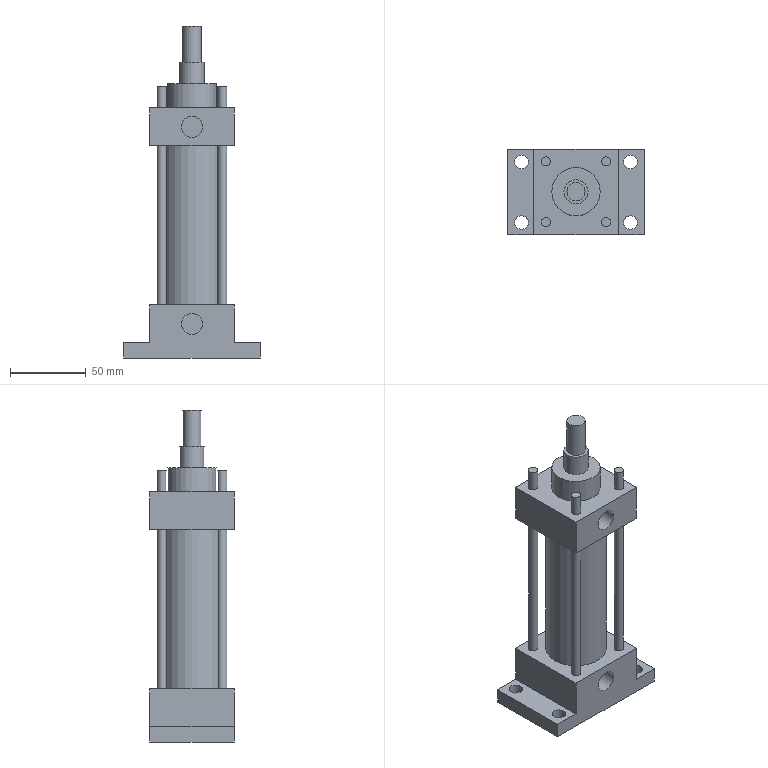Part | NX | features solid 2 | 1 solid | 48 faces | box 90 x 56 x 219 mm | volume 352785 mm3 | plane 28 | cylinder 20 | commonest cylinder face diameters 6 x8 9 x4 14 x2 7 x1 12 x1 16 x1
STEP:
#1=CARTESIAN_POINT('',(16.,-762.,-34.));
#2=VERTEX_POINT('',#1);
#3=CARTESIAN_POINT('',(0.,-762.,-34.));
#4=DIRECTION('',(0.,0.,1.));
#5=DIRECTION('',(1.,0.,0.));
#6=AXIS2_PLACEMENT_3D('',#3,#4,#5);
#7=CIRCLE('',#6,16.);
#8=EDGE_CURVE('',#2,#2,#7,.T.);
#9=ORIENTED_EDGE('',*,*,#8,.T.);
#10=EDGE_LOOP('',(#9));
#11=FACE_BOUND('',#10,.T.);
#12=CARTESIAN_POINT('',(8.,-762.,-34.));
#13=VERTEX_POINT('',#12);
#14=CARTESIAN_POINT('',(0.,-762.,-34.));
#15=DIRECTION('',(0.,0.,1.));
#16=DIRECTION('',(1.,0.,0.));
#17=AXIS2_PLACEMENT_3D('',#14,#15,#16);
#18=CIRCLE('',#17,8.);
#19=EDGE_CURVE('',#13,#13,#18,.F.);
#20=ORIENTED_EDGE('',*,*,#19,.T.);
#21=EDGE_LOOP('',(#20));
#22=FACE_BOUND('',#21,.T.);
#23=CARTESIAN_POINT('',(0.,-762.,-34.));
#24=DIRECTION('',(0.,0.,1.));
#25=DIRECTION('',(1.,0.,0.));
#26=AXIS2_PLACEMENT_3D('',#23,#24,#25);
#27=PLANE('',#26);
#28=ADVANCED_FACE('',(#11,#22),#27,.T.);
#29=CARTESIAN_POINT('',(-17.,-742.,-75.));
#30=VERTEX_POINT('',#29);
#31=CARTESIAN_POINT('',(-20.,-742.,-75.));
#32=DIRECTION('',(0.,0.,1.));
#33=DIRECTION('',(1.,0.,0.));
#34=AXIS2_PLACEMENT_3D('',#31,#32,#33);
#35=CIRCLE('',#34,3.);
#36=EDGE_CURVE('',#30,#30,#35,.T.);
#37=ORIENTED_EDGE('',*,*,#36,.T.);
#38=EDGE_LOOP('',(#37));
#39=FACE_BOUND('',#38,.T.);
#40=CARTESIAN_POINT('',(23.,-742.,-75.));
#41=VERTEX_POINT('',#40);
#42=CARTESIAN_POINT('',(20.,-742.,-75.));
#43=DIRECTION('',(0.,0.,1.));
#44=DIRECTION('',(1.,0.,0.));
#45=AXIS2_PLACEMENT_3D('',#42,#43,#44);
#46=CIRCLE('',#45,3.);
#47=EDGE_CURVE('',#41,#41,#46,.T.);
#48=ORIENTED_EDGE('',*,*,#47,.T.);
#49=EDGE_LOOP('',(#48));
#50=FACE_BOUND('',#49,.T.);
#51=CARTESIAN_POINT('',(23.,-782.,-75.));
#52=VERTEX_POINT('',#51);
#53=CARTESIAN_POINT('',(20.,-782.,-75.));
#54=DIRECTION('',(0.,0.,1.));
#55=DIRECTION('',(1.,0.,0.));
#56=AXIS2_PLACEMENT_3D('',#53,#54,#55);
#57=CIRCLE('',#56,3.);
#58=EDGE_CURVE('',#52,#52,#57,.T.);
#59=ORIENTED_EDGE('',*,*,#58,.T.);
#60=EDGE_LOOP('',(#59));
#61=FACE_BOUND('',#60,.T.);
#62=CARTESIAN_POINT('',(-17.,-782.,-75.));
#63=VERTEX_POINT('',#62);
#64=CARTESIAN_POINT('',(-20.,-782.,-75.));
#65=DIRECTION('',(0.,0.,1.));
#66=DIRECTION('',(1.,0.,0.));
#67=AXIS2_PLACEMENT_3D('',#64,#65,#66);
#68=CIRCLE('',#67,3.);
#69=EDGE_CURVE('',#63,#63,#68,.T.);
#70=ORIENTED_EDGE('',*,*,#69,.T.);
#71=EDGE_LOOP('',(#70));
#72=FACE_BOUND('',#71,.T.);
#73=CARTESIAN_POINT('',(-28.,-734.,-75.));
#74=VERTEX_POINT('',#73);
#75=CARTESIAN_POINT('',(28.,-734.,-75.));
#76=VERTEX_POINT('',#75);
#77=CARTESIAN_POINT('',(-28.,-734.,-75.));
#78=DIRECTION('',(1.,0.,0.));
#79=VECTOR('',#78,1000.);
#80=LINE('',#77,#79);
#81=EDGE_CURVE('',#74,#76,#80,.T.);
#82=ORIENTED_EDGE('',*,*,#81,.T.);
#83=CARTESIAN_POINT('',(28.,-790.,-75.));
#84=VERTEX_POINT('',#83);
#85=CARTESIAN_POINT('',(28.,-734.,-75.));
#86=DIRECTION('',(0.,-1.,0.));
#87=VECTOR('',#86,1000.);
#88=LINE('',#85,#87);
#89=EDGE_CURVE('',#76,#84,#88,.T.);
#90=ORIENTED_EDGE('',*,*,#89,.T.);
#91=CARTESIAN_POINT('',(-28.,-790.,-75.));
#92=VERTEX_POINT('',#91);
#93=CARTESIAN_POINT('',(28.,-790.,-75.));
#94=DIRECTION('',(-1.,0.,0.));
#95=VECTOR('',#94,1000.);
#96=LINE('',#93,#95);
#97=EDGE_CURVE('',#84,#92,#96,.T.);
#98=ORIENTED_EDGE('',*,*,#97,.T.);
#99=CARTESIAN_POINT('',(-28.,-790.,-75.));
#100=DIRECTION('',(0.,1.,0.));
#101=VECTOR('',#100,1000.);
#102=LINE('',#99,#101);
#103=EDGE_CURVE('',#92,#74,#102,.T.);
#104=ORIENTED_EDGE('',*,*,#103,.T.);
#105=EDGE_LOOP('',(#82,#90,#98,#104));
#106=FACE_BOUND('',#105,.T.);
#107=CARTESIAN_POINT('',(20.,-762.,-75.));
#108=VERTEX_POINT('',#107);
#109=CARTESIAN_POINT('',(0.,-762.,-75.));
#110=DIRECTION('',(0.,0.,1.));
#111=DIRECTION('',(1.,0.,0.));
#112=AXIS2_PLACEMENT_3D('',#109,#110,#111);
#113=CIRCLE('',#112,20.);
#114=EDGE_CURVE('',#108,#108,#113,.F.);
#115=ORIENTED_EDGE('',*,*,#114,.F.);
#116=EDGE_LOOP('',(#115));
#117=FACE_BOUND('',#116,.T.);
#118=CARTESIAN_POINT('',(-28.,-734.,-75.));
#119=DIRECTION('',(0.,0.,1.));
#120=DIRECTION('',(1.,0.,0.));
#121=AXIS2_PLACEMENT_3D('',#118,#119,#120);
#122=PLANE('',#121);
#123=ADVANCED_FACE('',(#39,#50,#61,#72,#106,#117),#122,.F.);
#124=ORIENTED_EDGE('',*,*,#8,.F.);
#125=EDGE_LOOP('',(#124));
#126=FACE_BOUND('',#125,.T.);
#127=CARTESIAN_POINT('',(16.,-762.,-50.));
#128=VERTEX_POINT('',#127);
#129=CARTESIAN_POINT('',(0.,-762.,-50.));
#130=DIRECTION('',(0.,0.,1.));
#131=DIRECTION('',(1.,0.,0.));
#132=AXIS2_PLACEMENT_3D('',#129,#130,#131);
#133=CIRCLE('',#132,16.);
#134=EDGE_CURVE('',#128,#128,#133,.T.);
#135=ORIENTED_EDGE('',*,*,#134,.T.);
#136=EDGE_LOOP('',(#135));
#137=FACE_BOUND('',#136,.T.);
#138=CARTESIAN_POINT('',(0.,-762.,-34.));
#139=DIRECTION('',(0.,0.,-1.));
#140=DIRECTION('',(-1.,0.,0.));
#141=AXIS2_PLACEMENT_3D('',#138,#139,#140);
#142=CYLINDRICAL_SURFACE('',#141,16.);
#143=ADVANCED_FACE('',(#126,#137),#142,.T.);
#144=CARTESIAN_POINT('',(-17.,-742.,-50.));
#145=VERTEX_POINT('',#144);
#146=CARTESIAN_POINT('',(-20.,-742.,-50.));
#147=DIRECTION('',(0.,0.,1.));
#148=DIRECTION('',(1.,0.,0.));
#149=AXIS2_PLACEMENT_3D('',#146,#147,#148);
#150=CIRCLE('',#149,3.);
#151=EDGE_CURVE('',#145,#145,#150,.T.);
#152=ORIENTED_EDGE('',*,*,#151,.F.);
#153=EDGE_LOOP('',(#152));
#154=FACE_BOUND('',#153,.T.);
#155=CARTESIAN_POINT('',(23.,-742.,-50.));
#156=VERTEX_POINT('',#155);
#157=CARTESIAN_POINT('',(20.,-742.,-50.));
#158=DIRECTION('',(0.,0.,1.));
#159=DIRECTION('',(1.,0.,0.));
#160=AXIS2_PLACEMENT_3D('',#157,#158,#159);
#161=CIRCLE('',#160,3.);
#162=EDGE_CURVE('',#156,#156,#161,.T.);
#163=ORIENTED_EDGE('',*,*,#162,.F.);
#164=EDGE_LOOP('',(#163));
#165=FACE_BOUND('',#164,.T.);
#166=CARTESIAN_POINT('',(23.,-782.,-50.));
#167=VERTEX_POINT('',#166);
#168=CARTESIAN_POINT('',(20.,-782.,-50.));
#169=DIRECTION('',(0.,0.,1.));
#170=DIRECTION('',(1.,0.,0.));
#171=AXIS2_PLACEMENT_3D('',#168,#169,#170);
#172=CIRCLE('',#171,3.);
#173=EDGE_CURVE('',#167,#167,#172,.T.);
#174=ORIENTED_EDGE('',*,*,#173,.F.);
#175=EDGE_LOOP('',(#174));
#176=FACE_BOUND('',#175,.T.);
#177=CARTESIAN_POINT('',(-17.,-782.,-50.));
#178=VERTEX_POINT('',#177);
#179=CARTESIAN_POINT('',(-20.,-782.,-50.));
#180=DIRECTION('',(0.,0.,1.));
#181=DIRECTION('',(1.,0.,0.));
#182=AXIS2_PLACEMENT_3D('',#179,#180,#181);
#183=CIRCLE('',#182,3.);
#184=EDGE_CURVE('',#178,#178,#183,.T.);
#185=ORIENTED_EDGE('',*,*,#184,.F.);
#186=EDGE_LOOP('',(#185));
#187=FACE_BOUND('',#186,.T.);
#188=ORIENTED_EDGE('',*,*,#134,.F.);
#189=EDGE_LOOP('',(#188));
#190=FACE_BOUND('',#189,.T.);
#191=CARTESIAN_POINT('',(-28.,-734.,-50.));
#192=VERTEX_POINT('',#191);
#193=CARTESIAN_POINT('',(28.,-734.,-50.));
#194=VERTEX_POINT('',#193);
#195=CARTESIAN_POINT('',(-28.,-734.,-50.));
#196=DIRECTION('',(1.,0.,0.));
#197=VECTOR('',#196,1000.);
#198=LINE('',#195,#197);
#199=EDGE_CURVE('',#192,#194,#198,.T.);
#200=ORIENTED_EDGE('',*,*,#199,.F.);
#201=CARTESIAN_POINT('',(-28.,-790.,-50.));
#202=VERTEX_POINT('',#201);
#203=CARTESIAN_POINT('',(-28.,-790.,-50.));
#204=DIRECTION('',(0.,1.,0.));
#205=VECTOR('',#204,1000.);
#206=LINE('',#203,#205);
#207=EDGE_CURVE('',#202,#192,#206,.T.);
#208=ORIENTED_EDGE('',*,*,#207,.F.);
#209=CARTESIAN_POINT('',(28.,-790.,-50.));
#210=VERTEX_POINT('',#209);
#211=CARTESIAN_POINT('',(28.,-790.,-50.));
#212=DIRECTION('',(-1.,0.,0.));
#213=VECTOR('',#212,1000.);
#214=LINE('',#211,#213);
#215=EDGE_CURVE('',#210,#202,#214,.T.);
#216=ORIENTED_EDGE('',*,*,#215,.F.);
#217=CARTESIAN_POINT('',(28.,-734.,-50.));
#218=DIRECTION('',(0.,-1.,0.));
#219=VECTOR('',#218,1000.);
#220=LINE('',#217,#219);
#221=EDGE_CURVE('',#194,#210,#220,.T.);
#222=ORIENTED_EDGE('',*,*,#221,.F.);
#223=EDGE_LOOP('',(#200,#208,#216,#222));
#224=FACE_BOUND('',#223,.T.);
#225=CARTESIAN_POINT('',(-28.,-734.,-50.));
#226=DIRECTION('',(0.,0.,1.));
#227=DIRECTION('',(1.,0.,0.));
#228=AXIS2_PLACEMENT_3D('',#225,#226,#227);
#229=PLANE('',#228);
#230=ADVANCED_FACE('',(#154,#165,#176,#187,#190,#224),#229,.T.);
#231=ORIENTED_EDGE('',*,*,#199,.T.);
#232=CARTESIAN_POINT('',(28.,-734.,-75.));
#233=DIRECTION('',(0.,0.,1.));
#234=VECTOR('',#233,1000.);
#235=LINE('',#232,#234);
#236=EDGE_CURVE('',#76,#194,#235,.T.);
#237=ORIENTED_EDGE('',*,*,#236,.F.);
#238=ORIENTED_EDGE('',*,*,#81,.F.);
#239=CARTESIAN_POINT('',(-28.,-734.,-75.));
#240=DIRECTION('',(0.,0.,1.));
#241=VECTOR('',#240,1000.);
#242=LINE('',#239,#241);
#243=EDGE_CURVE('',#74,#192,#242,.T.);
#244=ORIENTED_EDGE('',*,*,#243,.T.);
#245=EDGE_LOOP('',(#231,#237,#238,#244));
#246=FACE_BOUND('',#245,.T.);
#247=CARTESIAN_POINT('',(-28.,-734.,-75.));
#248=DIRECTION('',(0.,-1.,0.));
#249=DIRECTION('',(0.,0.,-1.));
#250=AXIS2_PLACEMENT_3D('',#247,#248,#249);
#251=PLANE('',#250);
#252=ADVANCED_FACE('',(#246),#251,.F.);
#253=ORIENTED_EDGE('',*,*,#221,.T.);
#254=CARTESIAN_POINT('',(28.,-790.,-75.));
#255=DIRECTION('',(0.,0.,1.));
#256=VECTOR('',#255,1000.);
#257=LINE('',#254,#256);
#258=EDGE_CURVE('',#84,#210,#257,.T.);
#259=ORIENTED_EDGE('',*,*,#258,.F.);
#260=ORIENTED_EDGE('',*,*,#89,.F.);
#261=ORIENTED_EDGE('',*,*,#236,.T.);
#262=EDGE_LOOP('',(#253,#259,#260,#261));
#263=FACE_BOUND('',#262,.T.);
#264=CARTESIAN_POINT('',(28.,-734.,-75.));
#265=DIRECTION('',(-1.,0.,0.));
#266=DIRECTION('',(0.,-1.,0.));
#267=AXIS2_PLACEMENT_3D('',#264,#265,#266);
#268=PLANE('',#267);
#269=ADVANCED_FACE('',(#263),#268,.F.);
#270=CARTESIAN_POINT('',(0.,-790.,-55.5));
#271=VERTEX_POINT('',#270);
#272=CARTESIAN_POINT('',(0.,-790.,-62.5));
#273=DIRECTION('',(0.,1.,0.));
#274=DIRECTION('',(0.,0.,1.));
#275=AXIS2_PLACEMENT_3D('',#272,#273,#274);
#276=CIRCLE('',#275,7.);
#277=EDGE_CURVE('',#271,#271,#276,.T.);
#278=ORIENTED_EDGE('',*,*,#277,.T.);
#279=EDGE_LOOP('',(#278));
#280=FACE_BOUND('',#279,.T.);
#281=ORIENTED_EDGE('',*,*,#215,.T.);
#282=CARTESIAN_POINT('',(-28.,-790.,-75.));
#283=DIRECTION('',(0.,0.,1.));
#284=VECTOR('',#283,1000.);
#285=LINE('',#282,#284);
#286=EDGE_CURVE('',#92,#202,#285,.T.);
#287=ORIENTED_EDGE('',*,*,#286,.F.);
#288=ORIENTED_EDGE('',*,*,#97,.F.);
#289=ORIENTED_EDGE('',*,*,#258,.T.);
#290=EDGE_LOOP('',(#281,#287,#288,#289));
#291=FACE_BOUND('',#290,.T.);
#292=CARTESIAN_POINT('',(28.,-790.,-75.));
#293=DIRECTION('',(0.,1.,0.));
#294=DIRECTION('',(-1.,0.,0.));
#295=AXIS2_PLACEMENT_3D('',#292,#293,#294);
#296=PLANE('',#295);
#297=ADVANCED_FACE('',(#280,#291),#296,.F.);
#298=ORIENTED_EDGE('',*,*,#207,.T.);
#299=ORIENTED_EDGE('',*,*,#243,.F.);
#300=ORIENTED_EDGE('',*,*,#103,.F.);
#301=ORIENTED_EDGE('',*,*,#286,.T.);
#302=EDGE_LOOP('',(#298,#299,#300,#301));
#303=FACE_BOUND('',#302,.T.);
#304=CARTESIAN_POINT('',(-28.,-790.,-75.));
#305=DIRECTION('',(1.,0.,0.));
#306=DIRECTION('',(0.,0.,-1.));
#307=AXIS2_PLACEMENT_3D('',#304,#305,#306);
#308=PLANE('',#307);
#309=ADVANCED_FACE('',(#303),#308,.F.);
#310=CARTESIAN_POINT('',(20.,-762.,-180.));
#311=VERTEX_POINT('',#310);
#312=CARTESIAN_POINT('',(0.,-762.,-180.));
#313=DIRECTION('',(0.,0.,1.));
#314=DIRECTION('',(1.,0.,0.));
#315=AXIS2_PLACEMENT_3D('',#312,#313,#314);
#316=CIRCLE('',#315,20.);
#317=EDGE_CURVE('',#311,#311,#316,.T.);
#318=ORIENTED_EDGE('',*,*,#317,.T.);
#319=EDGE_LOOP('',(#318));
#320=FACE_BOUND('',#319,.T.);
#321=ORIENTED_EDGE('',*,*,#114,.T.);
#322=EDGE_LOOP('',(#321));
#323=FACE_BOUND('',#322,.T.);
#324=CARTESIAN_POINT('',(0.,-762.,-50.));
#325=DIRECTION('',(0.,0.,-1.));
#326=DIRECTION('',(-1.,0.,0.));
#327=AXIS2_PLACEMENT_3D('',#324,#325,#326);
#328=CYLINDRICAL_SURFACE('',#327,20.);
#329=ADVANCED_FACE('',(#320,#323),#328,.T.);
#330=CARTESIAN_POINT('',(-28.,-790.,-180.));
#331=VERTEX_POINT('',#330);
#332=CARTESIAN_POINT('',(-28.,-734.,-180.));
#333=VERTEX_POINT('',#332);
#334=CARTESIAN_POINT('',(-28.,-790.,-180.));
#335=DIRECTION('',(0.,1.,0.));
#336=VECTOR('',#335,1000.);
#337=LINE('',#334,#336);
#338=EDGE_CURVE('',#331,#333,#337,.T.);
#339=ORIENTED_EDGE('',*,*,#338,.T.);
#340=CARTESIAN_POINT('',(-28.,-734.,-205.));
#341=VERTEX_POINT('',#340);
#342=CARTESIAN_POINT('',(-28.,-734.,-205.));
#343=DIRECTION('',(0.,0.,1.));
#344=VECTOR('',#343,1000.);
#345=LINE('',#342,#344);
#346=EDGE_CURVE('',#341,#333,#345,.T.);
#347=ORIENTED_EDGE('',*,*,#346,.F.);
#348=CARTESIAN_POINT('',(-28.,-790.,-205.));
#349=VERTEX_POINT('',#348);
#350=CARTESIAN_POINT('',(-28.,-790.,-205.));
#351=DIRECTION('',(0.,1.,0.));
#352=VECTOR('',#351,1000.);
#353=LINE('',#350,#352);
#354=EDGE_CURVE('',#349,#341,#353,.T.);
#355=ORIENTED_EDGE('',*,*,#354,.F.);
#356=CARTESIAN_POINT('',(-28.,-790.,-205.));
#357=DIRECTION('',(0.,0.,1.));
#358=VECTOR('',#357,1000.);
#359=LINE('',#356,#358);
#360=EDGE_CURVE('',#349,#331,#359,.T.);
#361=ORIENTED_EDGE('',*,*,#360,.T.);
#362=EDGE_LOOP('',(#339,#347,#355,#361));
#363=FACE_BOUND('',#362,.T.);
#364=CARTESIAN_POINT('',(-28.,-790.,-205.));
#365=DIRECTION('',(1.,0.,0.));
#366=DIRECTION('',(0.,0.,-1.));
#367=AXIS2_PLACEMENT_3D('',#364,#365,#366);
#368=PLANE('',#367);
#369=ADVANCED_FACE('',(#363),#368,.F.);
#370=CARTESIAN_POINT('',(0.,-790.,-185.5));
#371=VERTEX_POINT('',#370);
#372=CARTESIAN_POINT('',(0.,-790.,-192.5));
#373=DIRECTION('',(0.,1.,0.));
#374=DIRECTION('',(0.,0.,1.));
#375=AXIS2_PLACEMENT_3D('',#372,#373,#374);
#376=CIRCLE('',#375,7.);
#377=EDGE_CURVE('',#371,#371,#376,.T.);
#378=ORIENTED_EDGE('',*,*,#377,.T.);
#379=EDGE_LOOP('',(#378));
#380=FACE_BOUND('',#379,.T.);
#381=CARTESIAN_POINT('',(28.,-790.,-180.));
#382=VERTEX_POINT('',#381);
#383=CARTESIAN_POINT('',(28.,-790.,-180.));
#384=DIRECTION('',(-1.,0.,0.));
#385=VECTOR('',#384,1000.);
#386=LINE('',#383,#385);
#387=EDGE_CURVE('',#382,#331,#386,.T.);
#388=ORIENTED_EDGE('',*,*,#387,.T.);
#389=ORIENTED_EDGE('',*,*,#360,.F.);
#390=CARTESIAN_POINT('',(-45.,-790.,-205.));
#391=VERTEX_POINT('',#390);
#392=CARTESIAN_POINT('',(45.,-790.,-205.));
#393=DIRECTION('',(-1.,0.,0.));
#394=VECTOR('',#393,1000.);
#395=LINE('',#392,#394);
#396=EDGE_CURVE('',#349,#391,#395,.T.);
#397=ORIENTED_EDGE('',*,*,#396,.T.);
#398=CARTESIAN_POINT('',(-45.,-790.,-215.));
#399=VERTEX_POINT('',#398);
#400=CARTESIAN_POINT('',(-45.,-790.,-215.));
#401=DIRECTION('',(0.,0.,1.));
#402=VECTOR('',#401,1000.);
#403=LINE('',#400,#402);
#404=EDGE_CURVE('',#399,#391,#403,.T.);
#405=ORIENTED_EDGE('',*,*,#404,.F.);
#406=CARTESIAN_POINT('',(45.,-790.,-215.));
#407=VERTEX_POINT('',#406);
#408=CARTESIAN_POINT('',(45.,-790.,-215.));
#409=DIRECTION('',(-1.,0.,0.));
#410=VECTOR('',#409,1000.);
#411=LINE('',#408,#410);
#412=EDGE_CURVE('',#407,#399,#411,.T.);
#413=ORIENTED_EDGE('',*,*,#412,.F.);
#414=CARTESIAN_POINT('',(45.,-790.,-205.));
#415=VERTEX_POINT('',#414);
#416=CARTESIAN_POINT('',(45.,-790.,-215.));
#417=DIRECTION('',(0.,0.,1.));
#418=VECTOR('',#417,1000.);
#419=LINE('',#416,#418);
#420=EDGE_CURVE('',#407,#415,#419,.T.);
#421=ORIENTED_EDGE('',*,*,#420,.T.);
#422=CARTESIAN_POINT('',(28.,-790.,-205.));
#423=VERTEX_POINT('',#422);
#424=CARTESIAN_POINT('',(45.,-790.,-205.));
#425=DIRECTION('',(-1.,0.,0.));
#426=VECTOR('',#425,1000.);
#427=LINE('',#424,#426);
#428=EDGE_CURVE('',#415,#423,#427,.T.);
#429=ORIENTED_EDGE('',*,*,#428,.T.);
#430=CARTESIAN_POINT('',(28.,-790.,-205.));
#431=DIRECTION('',(0.,0.,1.));
#432=VECTOR('',#431,1000.);
#433=LINE('',#430,#432);
#434=EDGE_CURVE('',#423,#382,#433,.T.);
#435=ORIENTED_EDGE('',*,*,#434,.T.);
#436=EDGE_LOOP('',(#388,#389,#397,#405,#413,#421,#429,#435));
#437=FACE_BOUND('',#436,.T.);
#438=CARTESIAN_POINT('',(28.,-790.,-205.));
#439=DIRECTION('',(0.,1.,0.));
#440=DIRECTION('',(-1.,0.,0.));
#441=AXIS2_PLACEMENT_3D('',#438,#439,#440);
#442=PLANE('',#441);
#443=ADVANCED_FACE('',(#380,#437),#442,.F.);
#444=CARTESIAN_POINT('',(28.,-734.,-180.));
#445=VERTEX_POINT('',#444);
#446=CARTESIAN_POINT('',(28.,-734.,-180.));
#447=DIRECTION('',(0.,-1.,0.));
#448=VECTOR('',#447,1000.);
#449=LINE('',#446,#448);
#450=EDGE_CURVE('',#445,#382,#449,.T.);
#451=ORIENTED_EDGE('',*,*,#450,.T.);
#452=ORIENTED_EDGE('',*,*,#434,.F.);
#453=CARTESIAN_POINT('',(28.,-734.,-205.));
#454=VERTEX_POINT('',#453);
#455=CARTESIAN_POINT('',(28.,-734.,-205.));
#456=DIRECTION('',(0.,-1.,0.));
#457=VECTOR('',#456,1000.);
#458=LINE('',#455,#457);
#459=EDGE_CURVE('',#454,#423,#458,.T.);
#460=ORIENTED_EDGE('',*,*,#459,.F.);
#461=CARTESIAN_POINT('',(28.,-734.,-205.));
#462=DIRECTION('',(0.,0.,1.));
#463=VECTOR('',#462,1000.);
#464=LINE('',#461,#463);
#465=EDGE_CURVE('',#454,#445,#464,.T.);
#466=ORIENTED_EDGE('',*,*,#465,.T.);
#467=EDGE_LOOP('',(#451,#452,#460,#466));
#468=FACE_BOUND('',#467,.T.);
#469=CARTESIAN_POINT('',(28.,-734.,-205.));
#470=DIRECTION('',(-1.,0.,0.));
#471=DIRECTION('',(0.,-1.,0.));
#472=AXIS2_PLACEMENT_3D('',#469,#470,#471);
#473=PLANE('',#472);
#474=ADVANCED_FACE('',(#468),#473,.F.);
#475=CARTESIAN_POINT('',(-28.,-734.,-180.));
#476=DIRECTION('',(1.,0.,0.));
#477=VECTOR('',#476,1000.);
#478=LINE('',#475,#477);
#479=EDGE_CURVE('',#333,#445,#478,.T.);
#480=ORIENTED_EDGE('',*,*,#479,.T.);
#481=ORIENTED_EDGE('',*,*,#465,.F.);
#482=CARTESIAN_POINT('',(45.,-734.,-205.));
#483=VERTEX_POINT('',#482);
#484=CARTESIAN_POINT('',(-45.,-734.,-205.));
#485=DIRECTION('',(1.,0.,0.));
#486=VECTOR('',#485,1000.);
#487=LINE('',#484,#486);
#488=EDGE_CURVE('',#454,#483,#487,.T.);
#489=ORIENTED_EDGE('',*,*,#488,.T.);
#490=CARTESIAN_POINT('',(45.,-734.,-215.));
#491=VERTEX_POINT('',#490);
#492=CARTESIAN_POINT('',(45.,-734.,-215.));
#493=DIRECTION('',(0.,0.,1.));
#494=VECTOR('',#493,1000.);
#495=LINE('',#492,#494);
#496=EDGE_CURVE('',#491,#483,#495,.T.);
#497=ORIENTED_EDGE('',*,*,#496,.F.);
#498=CARTESIAN_POINT('',(-45.,-734.,-215.));
#499=VERTEX_POINT('',#498);
#500=CARTESIAN_POINT('',(-45.,-734.,-215.));
#501=DIRECTION('',(1.,0.,0.));
#502=VECTOR('',#501,1000.);
#503=LINE('',#500,#502);
#504=EDGE_CURVE('',#499,#491,#503,.T.);
#505=ORIENTED_EDGE('',*,*,#504,.F.);
#506=CARTESIAN_POINT('',(-45.,-734.,-205.));
#507=VERTEX_POINT('',#506);
#508=CARTESIAN_POINT('',(-45.,-734.,-215.));
#509=DIRECTION('',(0.,0.,1.));
#510=VECTOR('',#509,1000.);
#511=LINE('',#508,#510);
#512=EDGE_CURVE('',#499,#507,#511,.T.);
#513=ORIENTED_EDGE('',*,*,#512,.T.);
#514=CARTESIAN_POINT('',(-45.,-734.,-205.));
#515=DIRECTION('',(1.,0.,0.));
#516=VECTOR('',#515,1000.);
#517=LINE('',#514,#516);
#518=EDGE_CURVE('',#507,#341,#517,.T.);
#519=ORIENTED_EDGE('',*,*,#518,.T.);
#520=ORIENTED_EDGE('',*,*,#346,.T.);
#521=EDGE_LOOP('',(#480,#481,#489,#497,#505,#513,#519,#520));
#522=FACE_BOUND('',#521,.T.);
#523=CARTESIAN_POINT('',(-28.,-734.,-205.));
#524=DIRECTION('',(0.,-1.,0.));
#525=DIRECTION('',(0.,0.,-1.));
#526=AXIS2_PLACEMENT_3D('',#523,#524,#525);
#527=PLANE('',#526);
#528=ADVANCED_FACE('',(#522),#527,.F.);
#529=CARTESIAN_POINT('',(-17.,-742.,-180.));
#530=VERTEX_POINT('',#529);
#531=CARTESIAN_POINT('',(-20.,-742.,-180.));
#532=DIRECTION('',(0.,0.,1.));
#533=DIRECTION('',(1.,0.,0.));
#534=AXIS2_PLACEMENT_3D('',#531,#532,#533);
#535=CIRCLE('',#534,3.);
#536=EDGE_CURVE('',#530,#530,#535,.T.);
#537=ORIENTED_EDGE('',*,*,#536,.F.);
#538=EDGE_LOOP('',(#537));
#539=FACE_BOUND('',#538,.T.);
#540=CARTESIAN_POINT('',(23.,-742.,-180.));
#541=VERTEX_POINT('',#540);
#542=CARTESIAN_POINT('',(20.,-742.,-180.));
#543=DIRECTION('',(0.,0.,1.));
#544=DIRECTION('',(1.,0.,0.));
#545=AXIS2_PLACEMENT_3D('',#542,#543,#544);
#546=CIRCLE('',#545,3.);
#547=EDGE_CURVE('',#541,#541,#546,.T.);
#548=ORIENTED_EDGE('',*,*,#547,.F.);
#549=EDGE_LOOP('',(#548));
#550=FACE_BOUND('',#549,.T.);
#551=CARTESIAN_POINT('',(23.,-782.,-180.));
#552=VERTEX_POINT('',#551);
#553=CARTESIAN_POINT('',(20.,-782.,-180.));
#554=DIRECTION('',(0.,0.,1.));
#555=DIRECTION('',(1.,0.,0.));
#556=AXIS2_PLACEMENT_3D('',#553,#554,#555);
#557=CIRCLE('',#556,3.);
#558=EDGE_CURVE('',#552,#552,#557,.T.);
#559=ORIENTED_EDGE('',*,*,#558,.F.);
#560=EDGE_LOOP('',(#559));
#561=FACE_BOUND('',#560,.T.);
#562=CARTESIAN_POINT('',(-17.,-782.,-180.));
#563=VERTEX_POINT('',#562);
#564=CARTESIAN_POINT('',(-20.,-782.,-180.));
#565=DIRECTION('',(0.,0.,1.));
#566=DIRECTION('',(1.,0.,0.));
#567=AXIS2_PLACEMENT_3D('',#564,#565,#566);
#568=CIRCLE('',#567,3.);
#569=EDGE_CURVE('',#563,#563,#568,.T.);
#570=ORIENTED_EDGE('',*,*,#569,.F.);
#571=EDGE_LOOP('',(#570));
#572=FACE_BOUND('',#571,.T.);
#573=ORIENTED_EDGE('',*,*,#479,.F.);
#574=ORIENTED_EDGE('',*,*,#338,.F.);
#575=ORIENTED_EDGE('',*,*,#387,.F.);
#576=ORIENTED_EDGE('',*,*,#450,.F.);
#577=EDGE_LOOP('',(#573,#574,#575,#576));
#578=FACE_BOUND('',#577,.T.);
#579=ORIENTED_EDGE('',*,*,#317,.F.);
#580=EDGE_LOOP('',(#579));
#581=FACE_BOUND('',#580,.T.);
#582=CARTESIAN_POINT('',(-28.,-734.,-180.));
#583=DIRECTION('',(0.,0.,1.));
#584=DIRECTION('',(1.,0.,0.));
#585=AXIS2_PLACEMENT_3D('',#582,#583,#584);
#586=PLANE('',#585);
#587=ADVANCED_FACE('',(#539,#550,#561,#572,#578,#581),#586,.T.);
#588=CARTESIAN_POINT('',(31.5,-782.,-205.));
#589=VERTEX_POINT('',#588);
#590=CARTESIAN_POINT('',(36.,-782.,-205.));
#591=DIRECTION('',(0.,0.,-1.));
#592=DIRECTION('',(-1.,0.,0.));
#593=AXIS2_PLACEMENT_3D('',#590,#591,#592);
#594=CIRCLE('',#593,4.5);
#595=EDGE_CURVE('',#589,#589,#594,.T.);
#596=ORIENTED_EDGE('',*,*,#595,.T.);
#597=EDGE_LOOP('',(#596));
#598=FACE_BOUND('',#597,.T.);
#599=CARTESIAN_POINT('',(31.5,-742.,-205.));
#600=VERTEX_POINT('',#599);
#601=CARTESIAN_POINT('',(36.,-742.,-205.));
#602=DIRECTION('',(0.,0.,-1.));
#603=DIRECTION('',(-1.,0.,0.));
#604=AXIS2_PLACEMENT_3D('',#601,#602,#603);
#605=CIRCLE('',#604,4.5);
#606=EDGE_CURVE('',#600,#600,#605,.T.);
#607=ORIENTED_EDGE('',*,*,#606,.T.);
#608=EDGE_LOOP('',(#607));
#609=FACE_BOUND('',#608,.T.);
#610=ORIENTED_EDGE('',*,*,#488,.F.);
#611=ORIENTED_EDGE('',*,*,#459,.T.);
#612=ORIENTED_EDGE('',*,*,#428,.F.);
#613=CARTESIAN_POINT('',(45.,-734.,-205.));
#614=DIRECTION('',(0.,-1.,0.));
#615=VECTOR('',#614,1000.);
#616=LINE('',#613,#615);
#617=EDGE_CURVE('',#483,#415,#616,.T.);
#618=ORIENTED_EDGE('',*,*,#617,.F.);
#619=EDGE_LOOP('',(#610,#611,#612,#618));
#620=FACE_BOUND('',#619,.T.);
#621=CARTESIAN_POINT('',(45.,-734.,-205.));
#622=DIRECTION('',(0.,0.,-1.));
#623=DIRECTION('',(-1.,0.,0.));
#624=AXIS2_PLACEMENT_3D('',#621,#622,#623);
#625=PLANE('',#624);
#626=ADVANCED_FACE('',(#598,#609,#620),#625,.F.);
#627=CARTESIAN_POINT('',(-40.5,-782.,-205.));
#628=VERTEX_POINT('',#627);
#629=CARTESIAN_POINT('',(-36.,-782.,-205.));
#630=DIRECTION('',(0.,0.,-1.));
#631=DIRECTION('',(-1.,0.,0.));
#632=AXIS2_PLACEMENT_3D('',#629,#630,#631);
#633=CIRCLE('',#632,4.5);
#634=EDGE_CURVE('',#628,#628,#633,.T.);
#635=ORIENTED_EDGE('',*,*,#634,.T.);
#636=EDGE_LOOP('',(#635));
#637=FACE_BOUND('',#636,.T.);
#638=CARTESIAN_POINT('',(-40.5,-742.,-205.));
#639=VERTEX_POINT('',#638);
#640=CARTESIAN_POINT('',(-36.,-742.,-205.));
#641=DIRECTION('',(0.,0.,-1.));
#642=DIRECTION('',(-1.,0.,0.));
#643=AXIS2_PLACEMENT_3D('',#640,#641,#642);
#644=CIRCLE('',#643,4.5);
#645=EDGE_CURVE('',#639,#639,#644,.T.);
#646=ORIENTED_EDGE('',*,*,#645,.T.);
#647=EDGE_LOOP('',(#646));
#648=FACE_BOUND('',#647,.T.);
#649=ORIENTED_EDGE('',*,*,#396,.F.);
#650=ORIENTED_EDGE('',*,*,#354,.T.);
#651=ORIENTED_EDGE('',*,*,#518,.F.);
#652=CARTESIAN_POINT('',(-45.,-790.,-205.));
#653=DIRECTION('',(0.,1.,0.));
#654=VECTOR('',#653,1000.);
#655=LINE('',#652,#654);
#656=EDGE_CURVE('',#391,#507,#655,.T.);
#657=ORIENTED_EDGE('',*,*,#656,.F.);
#658=EDGE_LOOP('',(#649,#650,#651,#657));
#659=FACE_BOUND('',#658,.T.);
#660=CARTESIAN_POINT('',(45.,-734.,-205.));
#661=DIRECTION('',(0.,0.,-1.));
#662=DIRECTION('',(-1.,0.,0.));
#663=AXIS2_PLACEMENT_3D('',#660,#661,#662);
#664=PLANE('',#663);
#665=ADVANCED_FACE('',(#637,#648,#659),#664,.F.);
#666=ORIENTED_EDGE('',*,*,#617,.T.);
#667=ORIENTED_EDGE('',*,*,#420,.F.);
#668=CARTESIAN_POINT('',(45.,-734.,-215.));
#669=DIRECTION('',(0.,-1.,0.));
#670=VECTOR('',#669,1000.);
#671=LINE('',#668,#670);
#672=EDGE_CURVE('',#491,#407,#671,.T.);
#673=ORIENTED_EDGE('',*,*,#672,.F.);
#674=ORIENTED_EDGE('',*,*,#496,.T.);
#675=EDGE_LOOP('',(#666,#667,#673,#674));
#676=FACE_BOUND('',#675,.T.);
#677=CARTESIAN_POINT('',(45.,-734.,-215.));
#678=DIRECTION('',(-1.,0.,0.));
#679=DIRECTION('',(0.,0.,1.));
#680=AXIS2_PLACEMENT_3D('',#677,#678,#679);
#681=PLANE('',#680);
#682=ADVANCED_FACE('',(#676),#681,.F.);
#683=ORIENTED_EDGE('',*,*,#656,.T.);
#684=ORIENTED_EDGE('',*,*,#512,.F.);
#685=CARTESIAN_POINT('',(-45.,-790.,-215.));
#686=DIRECTION('',(0.,1.,0.));
#687=VECTOR('',#686,1000.);
#688=LINE('',#685,#687);
#689=EDGE_CURVE('',#399,#499,#688,.T.);
#690=ORIENTED_EDGE('',*,*,#689,.F.);
#691=ORIENTED_EDGE('',*,*,#404,.T.);
#692=EDGE_LOOP('',(#683,#684,#690,#691));
#693=FACE_BOUND('',#692,.T.);
#694=CARTESIAN_POINT('',(-45.,-790.,-215.));
#695=DIRECTION('',(1.,0.,0.));
#696=DIRECTION('',(0.,0.,-1.));
#697=AXIS2_PLACEMENT_3D('',#694,#695,#696);
#698=PLANE('',#697);
#699=ADVANCED_FACE('',(#693),#698,.F.);
#700=CARTESIAN_POINT('',(16.5,-762.,-215.));
#701=VERTEX_POINT('',#700);
#702=CARTESIAN_POINT('',(0.,-762.,-215.));
#703=DIRECTION('',(0.,0.,1.));
#704=DIRECTION('',(1.,0.,0.));
#705=AXIS2_PLACEMENT_3D('',#702,#703,#704);
#706=CIRCLE('',#705,16.5);
#707=EDGE_CURVE('',#701,#701,#706,.T.);
#708=ORIENTED_EDGE('',*,*,#707,.T.);
#709=EDGE_LOOP('',(#708));
#710=FACE_BOUND('',#709,.T.);
#711=CARTESIAN_POINT('',(40.5,-782.,-215.));
#712=VERTEX_POINT('',#711);
#713=CARTESIAN_POINT('',(36.,-782.,-215.));
#714=DIRECTION('',(0.,0.,1.));
#715=DIRECTION('',(1.,0.,0.));
#716=AXIS2_PLACEMENT_3D('',#713,#714,#715);
#717=CIRCLE('',#716,4.5);
#718=EDGE_CURVE('',#712,#712,#717,.T.);
#719=ORIENTED_EDGE('',*,*,#718,.T.);
#720=EDGE_LOOP('',(#719));
#721=FACE_BOUND('',#720,.T.);
#722=CARTESIAN_POINT('',(40.5,-742.,-215.));
#723=VERTEX_POINT('',#722);
#724=CARTESIAN_POINT('',(36.,-742.,-215.));
#725=DIRECTION('',(0.,0.,1.));
#726=DIRECTION('',(1.,0.,0.));
#727=AXIS2_PLACEMENT_3D('',#724,#725,#726);
#728=CIRCLE('',#727,4.5);
#729=EDGE_CURVE('',#723,#723,#728,.T.);
#730=ORIENTED_EDGE('',*,*,#729,.T.);
#731=EDGE_LOOP('',(#730));
#732=FACE_BOUND('',#731,.T.);
#733=CARTESIAN_POINT('',(-31.5,-782.,-215.));
#734=VERTEX_POINT('',#733);
#735=CARTESIAN_POINT('',(-36.,-782.,-215.));
#736=DIRECTION('',(0.,0.,1.));
#737=DIRECTION('',(1.,0.,0.));
#738=AXIS2_PLACEMENT_3D('',#735,#736,#737);
#739=CIRCLE('',#738,4.5);
#740=EDGE_CURVE('',#734,#734,#739,.T.);
#741=ORIENTED_EDGE('',*,*,#740,.T.);
#742=EDGE_LOOP('',(#741));
#743=FACE_BOUND('',#742,.T.);
#744=CARTESIAN_POINT('',(-31.5,-742.,-215.));
#745=VERTEX_POINT('',#744);
#746=CARTESIAN_POINT('',(-36.,-742.,-215.));
#747=DIRECTION('',(0.,0.,1.));
#748=DIRECTION('',(1.,0.,0.));
#749=AXIS2_PLACEMENT_3D('',#746,#747,#748);
#750=CIRCLE('',#749,4.5);
#751=EDGE_CURVE('',#745,#745,#750,.T.);
#752=ORIENTED_EDGE('',*,*,#751,.T.);
#753=EDGE_LOOP('',(#752));
#754=FACE_BOUND('',#753,.T.);
#755=ORIENTED_EDGE('',*,*,#504,.T.);
#756=ORIENTED_EDGE('',*,*,#672,.T.);
#757=ORIENTED_EDGE('',*,*,#412,.T.);
#758=ORIENTED_EDGE('',*,*,#689,.T.);
#759=EDGE_LOOP('',(#755,#756,#757,#758));
#760=FACE_BOUND('',#759,.T.);
#761=CARTESIAN_POINT('',(45.,-734.,-215.));
#762=DIRECTION('',(0.,0.,-1.));
#763=DIRECTION('',(-1.,0.,0.));
#764=AXIS2_PLACEMENT_3D('',#761,#762,#763);
#765=PLANE('',#764);
#766=ADVANCED_FACE('',(#710,#721,#732,#743,#754,#760),#765,.T.);
#767=CARTESIAN_POINT('',(8.,-762.,-20.));
#768=VERTEX_POINT('',#767);
#769=CARTESIAN_POINT('',(0.,-762.,-20.));
#770=DIRECTION('',(0.,0.,1.));
#771=DIRECTION('',(1.,0.,0.));
#772=AXIS2_PLACEMENT_3D('',#769,#770,#771);
#773=CIRCLE('',#772,8.);
#774=EDGE_CURVE('',#768,#768,#773,.T.);
#775=ORIENTED_EDGE('',*,*,#774,.T.);
#776=EDGE_LOOP('',(#775));
#777=FACE_BOUND('',#776,.T.);
#778=CARTESIAN_POINT('',(6.,-762.,-20.));
#779=VERTEX_POINT('',#778);
#780=CARTESIAN_POINT('',(0.,-762.,-20.));
#781=DIRECTION('',(0.,0.,1.));
#782=DIRECTION('',(1.,0.,0.));
#783=AXIS2_PLACEMENT_3D('',#780,#781,#782);
#784=CIRCLE('',#783,6.);
#785=EDGE_CURVE('',#779,#779,#784,.T.);
#786=ORIENTED_EDGE('',*,*,#785,.F.);
#787=EDGE_LOOP('',(#786));
#788=FACE_BOUND('',#787,.T.);
#789=CARTESIAN_POINT('',(0.,-762.,-20.));
#790=DIRECTION('',(0.,0.,1.));
#791=DIRECTION('',(1.,0.,0.));
#792=AXIS2_PLACEMENT_3D('',#789,#790,#791);
#793=PLANE('',#792);
#794=ADVANCED_FACE('',(#777,#788),#793,.T.);
#795=ORIENTED_EDGE('',*,*,#19,.F.);
#796=EDGE_LOOP('',(#795));
#797=FACE_BOUND('',#796,.T.);
#798=ORIENTED_EDGE('',*,*,#774,.F.);
#799=EDGE_LOOP('',(#798));
#800=FACE_BOUND('',#799,.T.);
#801=CARTESIAN_POINT('',(0.,-762.,-20.));
#802=DIRECTION('',(0.,0.,-1.));
#803=DIRECTION('',(-1.,0.,0.));
#804=AXIS2_PLACEMENT_3D('',#801,#802,#803);
#805=CYLINDRICAL_SURFACE('',#804,8.);
#806=ADVANCED_FACE('',(#797,#800),#805,.T.);
#807=CARTESIAN_POINT('',(6.,-762.,4.));
#808=VERTEX_POINT('',#807);
#809=CARTESIAN_POINT('',(0.,-762.,4.));
#810=DIRECTION('',(0.,0.,1.));
#811=DIRECTION('',(1.,0.,0.));
#812=AXIS2_PLACEMENT_3D('',#809,#810,#811);
#813=CIRCLE('',#812,6.);
#814=EDGE_CURVE('',#808,#808,#813,.T.);
#815=ORIENTED_EDGE('',*,*,#814,.T.);
#816=EDGE_LOOP('',(#815));
#817=FACE_BOUND('',#816,.T.);
#818=CARTESIAN_POINT('',(0.,-762.,4.));
#819=DIRECTION('',(0.,0.,1.));
#820=DIRECTION('',(1.,0.,0.));
#821=AXIS2_PLACEMENT_3D('',#818,#819,#820);
#822=PLANE('',#821);
#823=ADVANCED_FACE('',(#817),#822,.T.);
#824=ORIENTED_EDGE('',*,*,#785,.T.);
#825=EDGE_LOOP('',(#824));
#826=FACE_BOUND('',#825,.T.);
#827=ORIENTED_EDGE('',*,*,#814,.F.);
#828=EDGE_LOOP('',(#827));
#829=FACE_BOUND('',#828,.T.);
#830=CARTESIAN_POINT('',(0.,-762.,4.));
#831=DIRECTION('',(0.,0.,-1.));
#832=DIRECTION('',(-1.,0.,0.));
#833=AXIS2_PLACEMENT_3D('',#830,#831,#832);
#834=CYLINDRICAL_SURFACE('',#833,6.);
#835=ADVANCED_FACE('',(#826,#829),#834,.T.);
#836=ORIENTED_EDGE('',*,*,#569,.T.);
#837=EDGE_LOOP('',(#836));
#838=FACE_BOUND('',#837,.T.);
#839=ORIENTED_EDGE('',*,*,#69,.F.);
#840=EDGE_LOOP('',(#839));
#841=FACE_BOUND('',#840,.T.);
#842=CARTESIAN_POINT('',(-20.,-782.,-180.));
#843=DIRECTION('',(0.,0.,1.));
#844=DIRECTION('',(1.,0.,0.));
#845=AXIS2_PLACEMENT_3D('',#842,#843,#844);
#846=CYLINDRICAL_SURFACE('',#845,3.);
#847=ADVANCED_FACE('',(#838,#841),#846,.T.);
#848=CARTESIAN_POINT('',(-17.,-782.,-36.));
#849=VERTEX_POINT('',#848);
#850=CARTESIAN_POINT('',(-20.,-782.,-36.));
#851=DIRECTION('',(0.,0.,1.));
#852=DIRECTION('',(1.,0.,0.));
#853=AXIS2_PLACEMENT_3D('',#850,#851,#852);
#854=CIRCLE('',#853,3.);
#855=EDGE_CURVE('',#849,#849,#854,.T.);
#856=ORIENTED_EDGE('',*,*,#855,.T.);
#857=EDGE_LOOP('',(#856));
#858=FACE_BOUND('',#857,.T.);
#859=CARTESIAN_POINT('',(-20.,-782.,-36.));
#860=DIRECTION('',(0.,0.,1.));
#861=DIRECTION('',(1.,0.,0.));
#862=AXIS2_PLACEMENT_3D('',#859,#860,#861);
#863=PLANE('',#862);
#864=ADVANCED_FACE('',(#858),#863,.T.);
#865=ORIENTED_EDGE('',*,*,#184,.T.);
#866=EDGE_LOOP('',(#865));
#867=FACE_BOUND('',#866,.T.);
#868=ORIENTED_EDGE('',*,*,#855,.F.);
#869=EDGE_LOOP('',(#868));
#870=FACE_BOUND('',#869,.T.);
#871=CARTESIAN_POINT('',(-20.,-782.,-180.));
#872=DIRECTION('',(0.,0.,1.));
#873=DIRECTION('',(1.,0.,0.));
#874=AXIS2_PLACEMENT_3D('',#871,#872,#873);
#875=CYLINDRICAL_SURFACE('',#874,3.);
#876=ADVANCED_FACE('',(#867,#870),#875,.T.);
#877=ORIENTED_EDGE('',*,*,#558,.T.);
#878=EDGE_LOOP('',(#877));
#879=FACE_BOUND('',#878,.T.);
#880=ORIENTED_EDGE('',*,*,#58,.F.);
#881=EDGE_LOOP('',(#880));
#882=FACE_BOUND('',#881,.T.);
#883=CARTESIAN_POINT('',(20.,-782.,-180.));
#884=DIRECTION('',(0.,0.,1.));
#885=DIRECTION('',(1.,0.,0.));
#886=AXIS2_PLACEMENT_3D('',#883,#884,#885);
#887=CYLINDRICAL_SURFACE('',#886,3.);
#888=ADVANCED_FACE('',(#879,#882),#887,.T.);
#889=CARTESIAN_POINT('',(23.,-782.,-36.));
#890=VERTEX_POINT('',#889);
#891=CARTESIAN_POINT('',(20.,-782.,-36.));
#892=DIRECTION('',(0.,0.,1.));
#893=DIRECTION('',(1.,0.,0.));
#894=AXIS2_PLACEMENT_3D('',#891,#892,#893);
#895=CIRCLE('',#894,3.);
#896=EDGE_CURVE('',#890,#890,#895,.T.);
#897=ORIENTED_EDGE('',*,*,#896,.T.);
#898=EDGE_LOOP('',(#897));
#899=FACE_BOUND('',#898,.T.);
#900=CARTESIAN_POINT('',(20.,-782.,-36.));
#901=DIRECTION('',(0.,0.,1.));
#902=DIRECTION('',(1.,0.,0.));
#903=AXIS2_PLACEMENT_3D('',#900,#901,#902);
#904=PLANE('',#903);
#905=ADVANCED_FACE('',(#899),#904,.T.);
#906=ORIENTED_EDGE('',*,*,#173,.T.);
#907=EDGE_LOOP('',(#906));
#908=FACE_BOUND('',#907,.T.);
#909=ORIENTED_EDGE('',*,*,#896,.F.);
#910=EDGE_LOOP('',(#909));
#911=FACE_BOUND('',#910,.T.);
#912=CARTESIAN_POINT('',(20.,-782.,-180.));
#913=DIRECTION('',(0.,0.,1.));
#914=DIRECTION('',(1.,0.,0.));
#915=AXIS2_PLACEMENT_3D('',#912,#913,#914);
#916=CYLINDRICAL_SURFACE('',#915,3.);
#917=ADVANCED_FACE('',(#908,#911),#916,.T.);
#918=ORIENTED_EDGE('',*,*,#547,.T.);
#919=EDGE_LOOP('',(#918));
#920=FACE_BOUND('',#919,.T.);
#921=ORIENTED_EDGE('',*,*,#47,.F.);
#922=EDGE_LOOP('',(#921));
#923=FACE_BOUND('',#922,.T.);
#924=CARTESIAN_POINT('',(20.,-742.,-180.));
#925=DIRECTION('',(0.,0.,1.));
#926=DIRECTION('',(1.,0.,0.));
#927=AXIS2_PLACEMENT_3D('',#924,#925,#926);
#928=CYLINDRICAL_SURFACE('',#927,3.);
#929=ADVANCED_FACE('',(#920,#923),#928,.T.);
#930=CARTESIAN_POINT('',(23.,-742.,-36.));
#931=VERTEX_POINT('',#930);
#932=CARTESIAN_POINT('',(20.,-742.,-36.));
#933=DIRECTION('',(0.,0.,1.));
#934=DIRECTION('',(1.,0.,0.));
#935=AXIS2_PLACEMENT_3D('',#932,#933,#934);
#936=CIRCLE('',#935,3.);
#937=EDGE_CURVE('',#931,#931,#936,.T.);
#938=ORIENTED_EDGE('',*,*,#937,.T.);
#939=EDGE_LOOP('',(#938));
#940=FACE_BOUND('',#939,.T.);
#941=CARTESIAN_POINT('',(20.,-742.,-36.));
#942=DIRECTION('',(0.,0.,1.));
#943=DIRECTION('',(1.,0.,0.));
#944=AXIS2_PLACEMENT_3D('',#941,#942,#943);
#945=PLANE('',#944);
#946=ADVANCED_FACE('',(#940),#945,.T.);
#947=ORIENTED_EDGE('',*,*,#162,.T.);
#948=EDGE_LOOP('',(#947));
#949=FACE_BOUND('',#948,.T.);
#950=ORIENTED_EDGE('',*,*,#937,.F.);
#951=EDGE_LOOP('',(#950));
#952=FACE_BOUND('',#951,.T.);
#953=CARTESIAN_POINT('',(20.,-742.,-180.));
#954=DIRECTION('',(0.,0.,1.));
#955=DIRECTION('',(1.,0.,0.));
#956=AXIS2_PLACEMENT_3D('',#953,#954,#955);
#957=CYLINDRICAL_SURFACE('',#956,3.);
#958=ADVANCED_FACE('',(#949,#952),#957,.T.);
#959=ORIENTED_EDGE('',*,*,#536,.T.);
#960=EDGE_LOOP('',(#959));
#961=FACE_BOUND('',#960,.T.);
#962=ORIENTED_EDGE('',*,*,#36,.F.);
#963=EDGE_LOOP('',(#962));
#964=FACE_BOUND('',#963,.T.);
#965=CARTESIAN_POINT('',(-20.,-742.,-180.));
#966=DIRECTION('',(0.,0.,1.));
#967=DIRECTION('',(1.,0.,0.));
#968=AXIS2_PLACEMENT_3D('',#965,#966,#967);
#969=CYLINDRICAL_SURFACE('',#968,3.);
#970=ADVANCED_FACE('',(#961,#964),#969,.T.);
#971=CARTESIAN_POINT('',(-17.,-742.,-36.));
#972=VERTEX_POINT('',#971);
#973=CARTESIAN_POINT('',(-20.,-742.,-36.));
#974=DIRECTION('',(0.,0.,1.));
#975=DIRECTION('',(1.,0.,0.));
#976=AXIS2_PLACEMENT_3D('',#973,#974,#975);
#977=CIRCLE('',#976,3.);
#978=EDGE_CURVE('',#972,#972,#977,.T.);
#979=ORIENTED_EDGE('',*,*,#978,.T.);
#980=EDGE_LOOP('',(#979));
#981=FACE_BOUND('',#980,.T.);
#982=CARTESIAN_POINT('',(-20.,-742.,-36.));
#983=DIRECTION('',(0.,0.,1.));
#984=DIRECTION('',(1.,0.,0.));
#985=AXIS2_PLACEMENT_3D('',#982,#983,#984);
#986=PLANE('',#985);
#987=ADVANCED_FACE('',(#981),#986,.T.);
#988=ORIENTED_EDGE('',*,*,#151,.T.);
#989=EDGE_LOOP('',(#988));
#990=FACE_BOUND('',#989,.T.);
#991=ORIENTED_EDGE('',*,*,#978,.F.);
#992=EDGE_LOOP('',(#991));
#993=FACE_BOUND('',#992,.T.);
#994=CARTESIAN_POINT('',(-20.,-742.,-180.));
#995=DIRECTION('',(0.,0.,1.));
#996=DIRECTION('',(1.,0.,0.));
#997=AXIS2_PLACEMENT_3D('',#994,#995,#996);
#998=CYLINDRICAL_SURFACE('',#997,3.);
#999=ADVANCED_FACE('',(#990,#993),#998,.T.);
#1000=ORIENTED_EDGE('',*,*,#751,.F.);
#1001=EDGE_LOOP('',(#1000));
#1002=FACE_BOUND('',#1001,.T.);
#1003=ORIENTED_EDGE('',*,*,#645,.F.);
#1004=EDGE_LOOP('',(#1003));
#1005=FACE_BOUND('',#1004,.T.);
#1006=CARTESIAN_POINT('',(-36.,-742.,-215.));
#1007=DIRECTION('',(0.,0.,1.));
#1008=DIRECTION('',(1.,0.,0.));
#1009=AXIS2_PLACEMENT_3D('',#1006,#1007,#1008);
#1010=CYLINDRICAL_SURFACE('',#1009,4.5);
#1011=ADVANCED_FACE('',(#1002,#1005),#1010,.F.);
#1012=ORIENTED_EDGE('',*,*,#740,.F.);
#1013=EDGE_LOOP('',(#1012));
#1014=FACE_BOUND('',#1013,.T.);
#1015=ORIENTED_EDGE('',*,*,#634,.F.);
#1016=EDGE_LOOP('',(#1015));
#1017=FACE_BOUND('',#1016,.T.);
#1018=CARTESIAN_POINT('',(-36.,-782.,-215.));
#1019=DIRECTION('',(0.,0.,1.));
#1020=DIRECTION('',(1.,0.,0.));
#1021=AXIS2_PLACEMENT_3D('',#1018,#1019,#1020);
#1022=CYLINDRICAL_SURFACE('',#1021,4.5);
#1023=ADVANCED_FACE('',(#1014,#1017),#1022,.F.);
#1024=ORIENTED_EDGE('',*,*,#729,.F.);
#1025=EDGE_LOOP('',(#1024));
#1026=FACE_BOUND('',#1025,.T.);
#1027=ORIENTED_EDGE('',*,*,#606,.F.);
#1028=EDGE_LOOP('',(#1027));
#1029=FACE_BOUND('',#1028,.T.);
#1030=CARTESIAN_POINT('',(36.,-742.,-215.));
#1031=DIRECTION('',(0.,0.,1.));
#1032=DIRECTION('',(1.,0.,0.));
#1033=AXIS2_PLACEMENT_3D('',#1030,#1031,#1032);
#1034=CYLINDRICAL_SURFACE('',#1033,4.5);
#1035=ADVANCED_FACE('',(#1026,#1029),#1034,.F.);
#1036=ORIENTED_EDGE('',*,*,#718,.F.);
#1037=EDGE_LOOP('',(#1036));
#1038=FACE_BOUND('',#1037,.T.);
#1039=ORIENTED_EDGE('',*,*,#595,.F.);
#1040=EDGE_LOOP('',(#1039));
#1041=FACE_BOUND('',#1040,.T.);
#1042=CARTESIAN_POINT('',(36.,-782.,-215.));
#1043=DIRECTION('',(0.,0.,1.));
#1044=DIRECTION('',(1.,0.,0.));
#1045=AXIS2_PLACEMENT_3D('',#1042,#1043,#1044);
#1046=CYLINDRICAL_SURFACE('',#1045,4.5);
#1047=ADVANCED_FACE('',(#1038,#1041),#1046,.F.);
#1048=CARTESIAN_POINT('',(16.5,-762.,-205.));
#1049=VERTEX_POINT('',#1048);
#1050=CARTESIAN_POINT('',(0.,-762.,-205.));
#1051=DIRECTION('',(0.,0.,1.));
#1052=DIRECTION('',(1.,0.,0.));
#1053=AXIS2_PLACEMENT_3D('',#1050,#1051,#1052);
#1054=CIRCLE('',#1053,16.5);
#1055=EDGE_CURVE('',#1049,#1049,#1054,.T.);
#1056=ORIENTED_EDGE('',*,*,#1055,.F.);
#1057=EDGE_LOOP('',(#1056));
#1058=FACE_BOUND('',#1057,.T.);
#1059=CARTESIAN_POINT('',(0.,-762.,-205.));
#1060=DIRECTION('',(0.,0.,1.));
#1061=DIRECTION('',(1.,0.,0.));
#1062=AXIS2_PLACEMENT_3D('',#1059,#1060,#1061);
#1063=PLANE('',#1062);
#1064=ADVANCED_FACE('',(#1058),#1063,.F.);
#1065=ORIENTED_EDGE('',*,*,#1055,.T.);
#1066=EDGE_LOOP('',(#1065));
#1067=FACE_BOUND('',#1066,.T.);
#1068=ORIENTED_EDGE('',*,*,#707,.F.);
#1069=EDGE_LOOP('',(#1068));
#1070=FACE_BOUND('',#1069,.T.);
#1071=CARTESIAN_POINT('',(0.,-762.,-215.));
#1072=DIRECTION('',(0.,0.,1.));
#1073=DIRECTION('',(1.,0.,0.));
#1074=AXIS2_PLACEMENT_3D('',#1071,#1072,#1073);
#1075=CYLINDRICAL_SURFACE('',#1074,16.5);
#1076=ADVANCED_FACE('',(#1067,#1070),#1075,.F.);
#1077=CARTESIAN_POINT('',(0.,-780.,-185.5));
#1078=VERTEX_POINT('',#1077);
#1079=CARTESIAN_POINT('',(0.,-780.,-192.5));
#1080=DIRECTION('',(0.,1.,0.));
#1081=DIRECTION('',(0.,0.,1.));
#1082=AXIS2_PLACEMENT_3D('',#1079,#1080,#1081);
#1083=CIRCLE('',#1082,7.);
#1084=EDGE_CURVE('',#1078,#1078,#1083,.T.);
#1085=ORIENTED_EDGE('',*,*,#1084,.F.);
#1086=EDGE_LOOP('',(#1085));
#1087=FACE_BOUND('',#1086,.T.);
#1088=CARTESIAN_POINT('',(0.,-780.,-192.5));
#1089=DIRECTION('',(0.,1.,0.));
#1090=DIRECTION('',(0.,0.,1.));
#1091=AXIS2_PLACEMENT_3D('',#1088,#1089,#1090);
#1092=PLANE('',#1091);
#1093=ADVANCED_FACE('',(#1087),#1092,.F.);
#1094=ORIENTED_EDGE('',*,*,#1084,.T.);
#1095=EDGE_LOOP('',(#1094));
#1096=FACE_BOUND('',#1095,.T.);
#1097=ORIENTED_EDGE('',*,*,#377,.F.);
#1098=EDGE_LOOP('',(#1097));
#1099=FACE_BOUND('',#1098,.T.);
#1100=CARTESIAN_POINT('',(0.,-790.,-192.5));
#1101=DIRECTION('',(0.,1.,0.));
#1102=DIRECTION('',(0.,0.,1.));
#1103=AXIS2_PLACEMENT_3D('',#1100,#1101,#1102);
#1104=CYLINDRICAL_SURFACE('',#1103,7.);
#1105=ADVANCED_FACE('',(#1096,#1099),#1104,.F.);
#1106=CARTESIAN_POINT('',(0.,-780.,-55.5));
#1107=VERTEX_POINT('',#1106);
#1108=CARTESIAN_POINT('',(0.,-780.,-62.5));
#1109=DIRECTION('',(0.,1.,0.));
#1110=DIRECTION('',(0.,0.,1.));
#1111=AXIS2_PLACEMENT_3D('',#1108,#1109,#1110);
#1112=CIRCLE('',#1111,7.);
#1113=EDGE_CURVE('',#1107,#1107,#1112,.T.);
#1114=ORIENTED_EDGE('',*,*,#1113,.F.);
#1115=EDGE_LOOP('',(#1114));
#1116=FACE_BOUND('',#1115,.T.);
#1117=CARTESIAN_POINT('',(0.,-780.,-62.5));
#1118=DIRECTION('',(0.,1.,0.));
#1119=DIRECTION('',(0.,0.,1.));
#1120=AXIS2_PLACEMENT_3D('',#1117,#1118,#1119);
#1121=PLANE('',#1120);
#1122=ADVANCED_FACE('',(#1116),#1121,.F.);
#1123=ORIENTED_EDGE('',*,*,#1113,.T.);
#1124=EDGE_LOOP('',(#1123));
#1125=FACE_BOUND('',#1124,.T.);
#1126=ORIENTED_EDGE('',*,*,#277,.F.);
#1127=EDGE_LOOP('',(#1126));
#1128=FACE_BOUND('',#1127,.T.);
#1129=CARTESIAN_POINT('',(0.,-790.,-62.5));
#1130=DIRECTION('',(0.,1.,0.));
#1131=DIRECTION('',(0.,0.,1.));
#1132=AXIS2_PLACEMENT_3D('',#1129,#1130,#1131);
#1133=CYLINDRICAL_SURFACE('',#1132,7.);
#1134=ADVANCED_FACE('',(#1125,#1128),#1133,.F.);
#1135=CLOSED_SHELL('',(#28,#123,#143,#230,#252,#269,#297,#309,#329,#369,#443,#474,#528,#587,#626,#665,#682,#699,#766,#794,#806,#823,#835,#847,#864,#876,#888,#905,#917,#929,#946,#958,#970,#987,#999,#1011,#1023,#1035,#1047,#1064,#1076,#1093,#1105,#1122,#1134));
#1136=CARTESIAN_POINT('',(3.5,-762.,-180.));
#1137=VERTEX_POINT('',#1136);
#1138=CARTESIAN_POINT('',(0.,-762.,-180.));
#1139=DIRECTION('',(0.,0.,1.));
#1140=DIRECTION('',(1.,0.,0.));
#1141=AXIS2_PLACEMENT_3D('',#1138,#1139,#1140);
#1142=CIRCLE('',#1141,3.5);
#1143=EDGE_CURVE('',#1137,#1137,#1142,.T.);
#1144=ORIENTED_EDGE('',*,*,#1143,.T.);
#1145=EDGE_LOOP('',(#1144));
#1146=FACE_BOUND('',#1145,.T.);
#1147=CARTESIAN_POINT('',(-28.,-734.,-180.));
#1148=DIRECTION('',(0.,0.,1.));
#1149=DIRECTION('',(1.,0.,0.));
#1150=AXIS2_PLACEMENT_3D('',#1147,#1148,#1149);
#1151=PLANE('',#1150);
#1152=ADVANCED_FACE('',(#1146),#1151,.T.);
#1153=CARTESIAN_POINT('',(3.5,-762.,-75.));
#1154=VERTEX_POINT('',#1153);
#1155=CARTESIAN_POINT('',(0.,-762.,-75.));
#1156=DIRECTION('',(0.,0.,1.));
#1157=DIRECTION('',(1.,0.,0.));
#1158=AXIS2_PLACEMENT_3D('',#1155,#1156,#1157);
#1159=CIRCLE('',#1158,3.5);
#1160=EDGE_CURVE('',#1154,#1154,#1159,.F.);
#1161=ORIENTED_EDGE('',*,*,#1160,.T.);
#1162=EDGE_LOOP('',(#1161));
#1163=FACE_BOUND('',#1162,.T.);
#1164=CARTESIAN_POINT('',(-28.,-734.,-75.));
#1165=DIRECTION('',(0.,0.,1.));
#1166=DIRECTION('',(1.,0.,0.));
#1167=AXIS2_PLACEMENT_3D('',#1164,#1165,#1166);
#1168=PLANE('',#1167);
#1169=ADVANCED_FACE('',(#1163),#1168,.F.);
#1170=ORIENTED_EDGE('',*,*,#1143,.F.);
#1171=EDGE_LOOP('',(#1170));
#1172=FACE_BOUND('',#1171,.T.);
#1173=ORIENTED_EDGE('',*,*,#1160,.F.);
#1174=EDGE_LOOP('',(#1173));
#1175=FACE_BOUND('',#1174,.T.);
#1176=CARTESIAN_POINT('',(0.,-762.,-50.));
#1177=DIRECTION('',(0.,0.,-1.));
#1178=DIRECTION('',(-1.,0.,0.));
#1179=AXIS2_PLACEMENT_3D('',#1176,#1177,#1178);
#1180=CYLINDRICAL_SURFACE('',#1179,3.5);
#1181=ADVANCED_FACE('',(#1172,#1175),#1180,.F.);
#1182=CLOSED_SHELL('',(#1152,#1169,#1181));
#1183=ORIENTED_CLOSED_SHELL('',*,#1182,.F.);
#1184=BREP_WITH_VOIDS('',#1135,(#1183));
#1185=(LENGTH_UNIT()NAMED_UNIT(*)SI_UNIT(.MILLI.,.METRE.));
#1186=UNCERTAINTY_MEASURE_WITH_UNIT(LENGTH_MEASURE(0.00001),#1185,'','');
#1187=(NAMED_UNIT(*)PLANE_ANGLE_UNIT()SI_UNIT($,.RADIAN.));
#1188=(NAMED_UNIT(*)SI_UNIT($,.STERADIAN.)SOLID_ANGLE_UNIT());
#1189=(GEOMETRIC_REPRESENTATION_CONTEXT(3)GLOBAL_UNCERTAINTY_ASSIGNED_CONTEXT((#1186))GLOBAL_UNIT_ASSIGNED_CONTEXT((#1185,#1187,#1188))REPRESENTATION_CONTEXT('',''));
#1190=ADVANCED_BREP_SHAPE_REPRESENTATION('',(#1184),#1189);